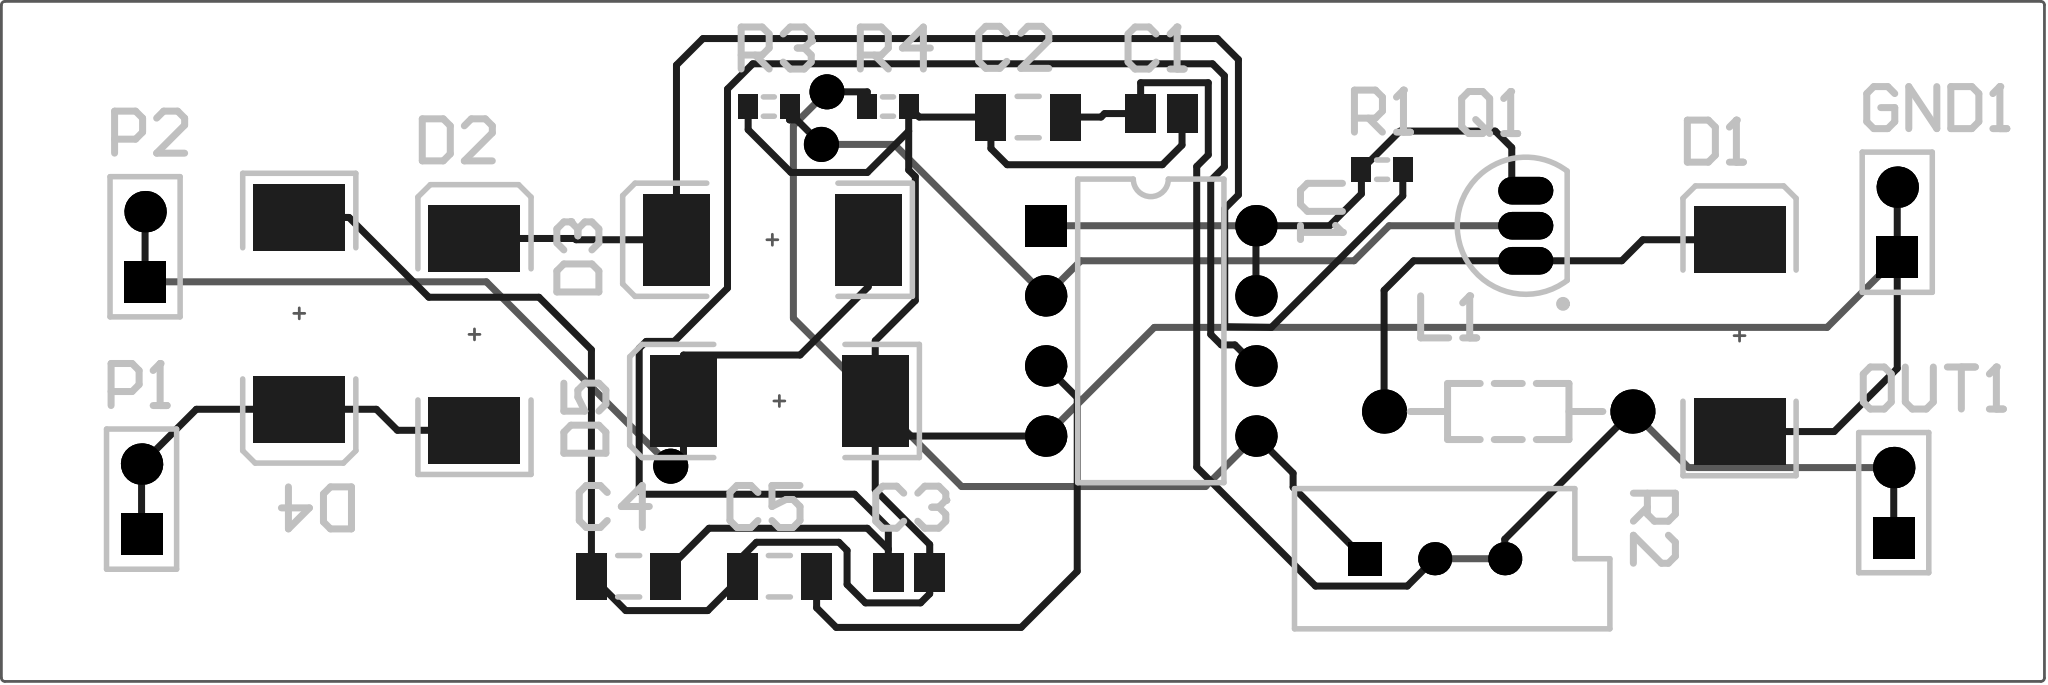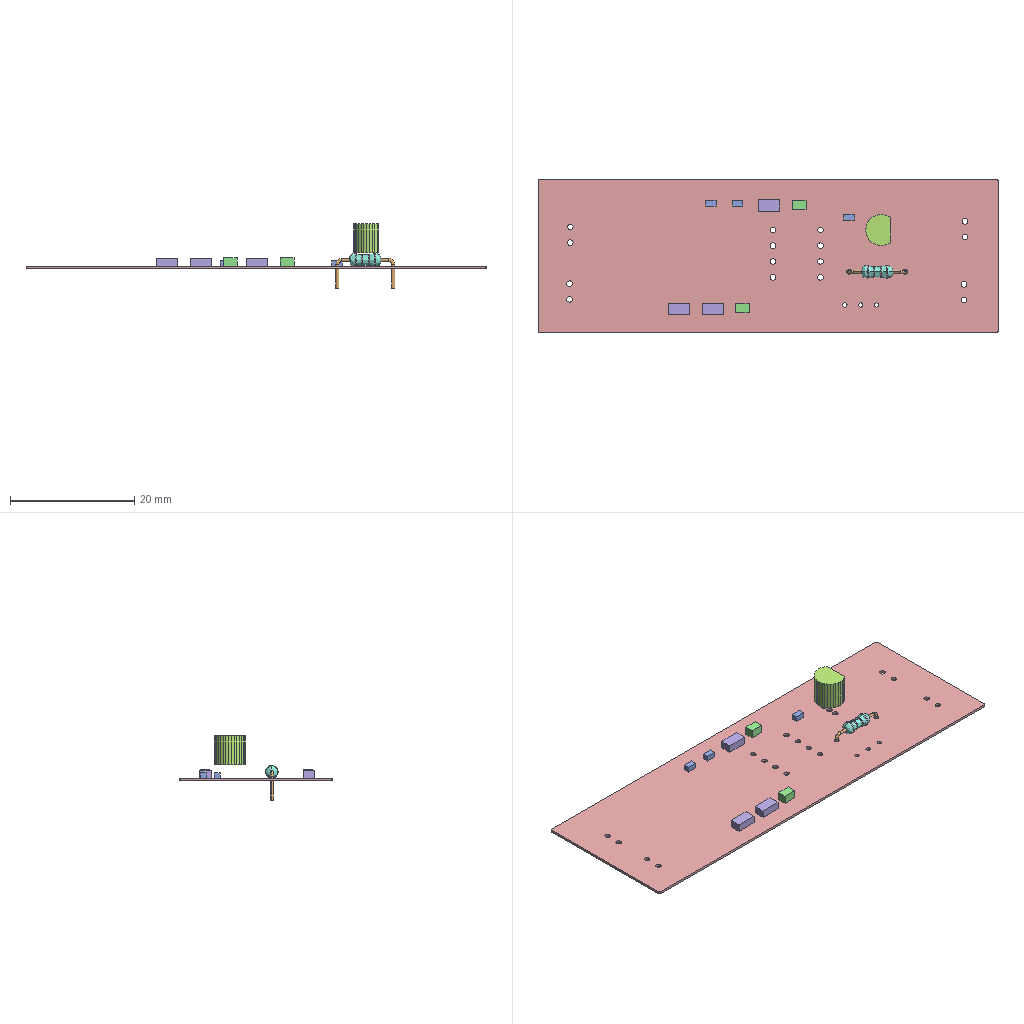Circuit board layout | Altium Designer | box 74 x 24.6 x 10.4 mm
Layer stack:
# Altium Designer layer stack of  (unit mm; dielectric type: 0 none, 1 core, 2 prepreg, 3 surface material)
index,name,kind,layer,copper_thickness_mm,dielectric_type,dielectric_thickness_mm,dielectric_material,dielectric_constant
0,Top Paste,other,,,,,,
1,Top Overlay,other,,,,,,
2,Top Solder,dielectric,,,3,0.0102,Solder Resist,3.5
3,Top Layer,copper,Top Layer,0.0356,,,,
4,Dielectric 1,dielectric,,,0,0.32,FR-4,4.8
5,Bottom Layer,copper,Bottom Layer,0.0356,,,,
6,Bottom Solder,dielectric,,,3,0.0102,Solder Resist,3.5
7,Bottom Overlay,other,,,,,,
8,Bottom Paste,other,,,,,,
# drill layer pairs: low layer,high layer
drill_pair,Top Layer,Bottom Layer
Part placement:
Designator,Comment,Layer,Footprint,Center-X(mm),Center-Y(mm),Rotation
U1,MC34063,TopLayer,693-02,103.251,77.089,270
R4,3.3K,TopLayer,J1-0603,93.726,85.217,0
R3,2K,TopLayer,J1-0603,89.408,85.217,0
R2,RPot,TopLayer,VR5,113.538,68.834,360
R1,0.1,TopLayer,J1-0603,111.633,82.931,360
Q1,2N3904,TopLayer,TO-92A,116.84,80.899,360
P2,Header 2,TopLayer,HDR1X2,66.802,80.137,90
P1,Header 2,TopLayer,HDR1X2,66.675,70.993,90
OUT1,Header 2,TopLayer,HDR1X2,130.175,70.866,90
L1,470UH,TopLayer,AL0204,116.205,74.168,360
GND1,Header 2,TopLayer,HDR1X2,130.302,81.026,90
D5,Diode,TopLayer,SMC,89.789,74.549,180
D4,Diode,TopLayer,SMC,72.39,77.724,270
D3,Diode,TopLayer,SMC,89.535,80.391,180
D2,Diode,TopLayer,SMC,78.74,76.962,90
D1,Diode,TopLayer,SMC,124.587,76.916,90
C5,180U,TopLayer,C1206,89.789,68.199,0
C4,104,TopLayer,C1206,84.328,68.199,0
C3,470U,TopLayer,C0805,94.488,68.326,0
C2,104,TopLayer,C1206,98.806,84.836,0
C1,1000UF,TopLayer,C0805,103.632,84.963,0
Pad and via stacks:
# Altium Designer via and pad stacks of  (unit mm). Each distinct definition once, with the count of objects using it.
# via: kind,start_layer,end_layer,hole_mm,diameter_mm,mode(0 simple;1 top-mid-bottom;2 full stack),diameter_per_layer,count,example_net
# pad: kind,layer,hole_mm,hole_type(0 round;1 square;2 slot),plating,top_size,top_shape(1 round;2 rect;3 octagon;9 rounded rect),mid_size,bottom_size,mode,footprint,size_per_layer,count,example
pad,Top Layer,0,0,plated,0.9x0.7,2,0.9x0.7,0.9x0.7,0,J1-0603,,6,R1.1
pad,Top Layer,0,0,plated,2.4x3.3,2,2.4x3.3,2.4x3.3,0,SMC,,10,D1.1
pad,Top Layer,0,0,plated,1.4x1.1,2,1.4x1.1,1.4x1.1,0,C0805,,4,C1.2
pad,Top Layer,0,0,plated,1.7x1.1,2,1.7x1.1,1.7x1.1,0,C1206,,6,C2.2
pad,Multi-Layer,0.8,0,plated,1.6x1.6,1,1.6x1.6,1.6x1.6,0,AL0204,,2,L1.2
pad,Multi-Layer,0.9,0,plated,2x1,1,2x1,2x1,0,TO-92A,,3,Q1.3
pad,Multi-Layer,0.9,0,plated,1.5x1.5,1,1.5x1.5,1.5x1.5,0,693-02,,7,U1.5
pad,Multi-Layer,0.9,0,plated,1.5x1.5,2,1.5x1.5,1.5x1.5,0,693-02,,1,U1.1
pad,Multi-Layer,0.9,0,plated,1.5x1.5,2,1.5x1.5,1.5x1.5,0,HDR1X2,,4,P1.1
pad,Multi-Layer,0.9,0,plated,1.5x1.5,1,1.5x1.5,1.5x1.5,0,HDR1X2,,4,P1.2
pad,Multi-Layer,0.7,0,plated,1.2x1.2,2,1.2x1.2,1.2x1.2,0,VR5,,1,R2.1
pad,Multi-Layer,0.7,0,plated,1.2x1.2,1,1.2x1.2,1.2x1.2,0,VR5,,2,R2.2
via,Top Layer,Bottom Layer,0.7112,1.27,0,,3,NetQ1_2
Design rules, without the lines most boards share:
# Altium Designer design rules of  (exported by Altium Designer, unit mm)
# columns: name | kind | enabled | priority | scope1 | scope2 | descriptor | typed fields (field=value)
HoleToHoleClearance | 52 | enabled | 1 | All | All | Hole To Hole Clearance (Gap=10mil) (All),(All) | gap=0.254
DiffPairsRouting | 51 | enabled | 1 | All | All | Differential Pairs Uncoupled Length using the Gap Constraints (Min=10mil) (Max=10mil) (Prefered=10mil)  and Width Constraints (Min=15mil) (Max=15mil) (Prefered=15mil) (All) |
SolderMaskExpansion | 13 | enabled | 1 | All | All | Solder Mask Expansion (Expansion =4mil) (All) | expansion=0.1016
PasteMaskExpansion | 14 | enabled | 1 | All | All | Paste Mask Expansion (Expansion =0mil) (All) | expansion=0
RoutingVias | 11 | enabled | 1 | All | All | Routing Via (MinHoleWidth=28mil) (MaxHoleWidth=28mil) (PreferredHoleWidth=28mil) (MinWidth=50mil) (MaxWidth=50mil) (PreferedWidth=50mil) (All) | via_min_hole=0.7112 via_max_hole=0.7112 via_preferred_diameter=1.27 via_preferred_hole=0.7112
Width | 2 | enabled | 1 | All | All | Width Constraint (Min=10mil) (Max=10mil) (Preferred=10mil) (All) |
PolygonConnect | 20 | enabled | 1 | All | All | Polygon Connect Rule(Relief Connect )(Conductor Width=10mil) (Relief Angle=90 Angle) (Entries=4) (Air Gap Width=10mil) (All),(All) | connect_style(0=relief,1=direct,2=none)=0 relief_conductor_width=0.254 relief_entries=4
PlaneConnect | 6 | enabled | 1 | All | All | Power Plane Connect Rule(Relief Connect )(Expansion=20mil) (Conductor Width=10mil) (Air Gap=10mil) (Entries=4) (All) | relief_conductor_width=0.254 relief_entries=4 relief_expansion=0.508
Clearance | 0 | enabled | 1 | All | All | Clearance Constraint (Gap=10mil) (All),(All) | gap=0.254
Classes set for this board:
# Altium Designer classes of  (member kind: 0 net, 1 component, 2 from-to, 3 pad, 4 layer, 5 differential pair, 6 design channel, 7 polygon, 8 structure, 9 xSignal)
# columns: class name | member kind | superclass | members
Sheet2 | 1 | no | C1; C2; C3; C4; C5; D1; D2; D3; D4; D5; GND1; L1; OUT1; P1; P2; Q1; R1; R2; R3; R4; U1;